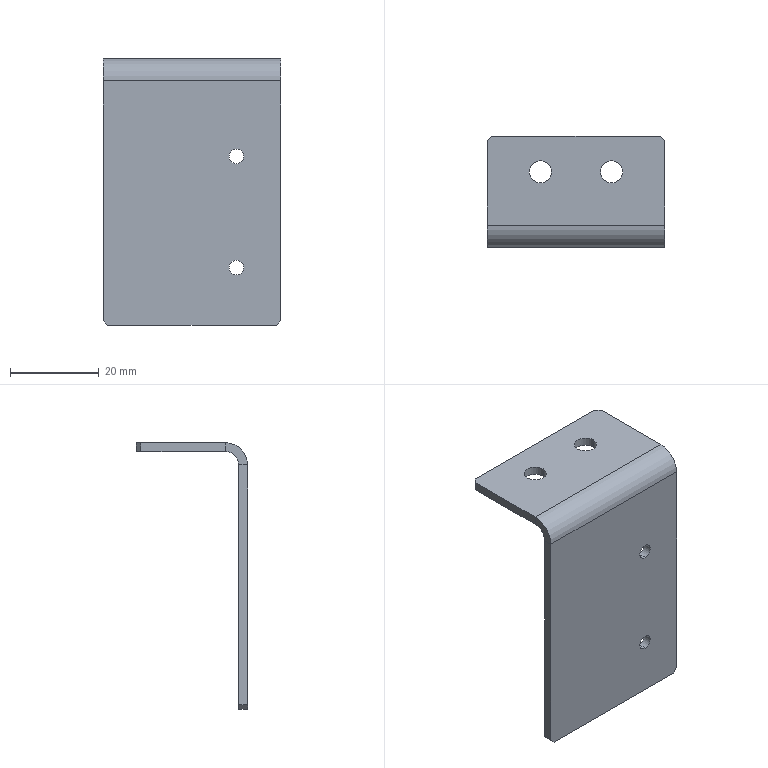Part | STEP file | 227H056254 BKT_Default | 1 solid | 26 faces | box 40 x 25 x 60 mm | volume 6386 mm3 | plane 16 | cylinder 10 | commonest cylinder face diameters 3.3 x4 5 x4 6 x1 10 x1